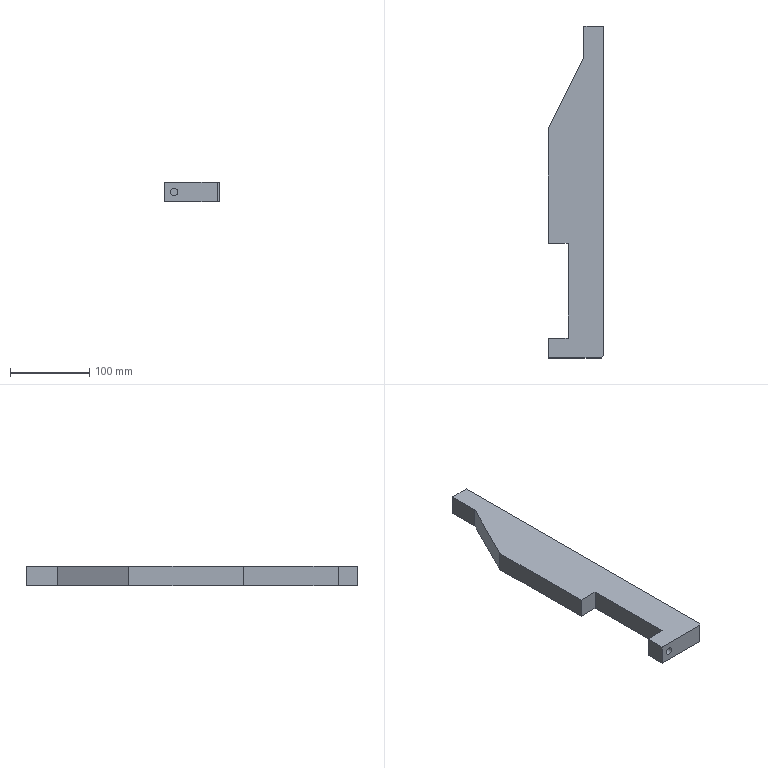CAM job | NX | 3-axis milling | part box 70 x 420 x 25 mm | stock box 75 x 425 x 30 mm
Tools:
number,name,description,diameter,corner_radius,flute_length,length,flutes
9,D10,平底铣刀-粗,10.0,0.0,35.0,75.0,2
11,D3-J,平底铣刀-精,3.0,0.0,50.0,75.0,2
7,D6-J,平底铣刀-精,6.0,0.0,25.0,75.0,2
1,D80R0.8飞刀,圆鼻刀-粗,80.0,0.8,50.0,75.0,2
1,D80R0.8飞刀-J,圆鼻刀-精,80.0,0.8,50.0,75.0,2
2,D6倒角刀,倒角刀,6.0,0.0,3.0,25.0,2
Operations:
program,operation,operation_type,tool,method,geometry_group,spindle_rpm,surface_speed,feed_per_tooth,feed_cut,feed_plunge,cut_length_mm,path_length_mm,cut_time_min,machine_time_min
B,FLOORWALL_FACE_ONEPASSROUGH_COPY,VolumeBased25DMillingOperation,D80R0.8飞刀,LAYERED-ROUGHING-DEPTHK-STEPG,W-B,2800.0,703.696,0.5357,3000.0,100.0,4753.746,9505.965,1.585,2.06
B,FLOORWALL_FACE_ONEPASSFINISH_COPY,VolumeBased25DMillingOperation,D80R0.8飞刀-J,SIDEWALL-FINISHING-DEPTHK-STEPG,W-B,4000.0,1005.28,0.125,1000.0,100.0,527.998,623.998,0.528,0.5376
B,PLANEDEBURR6X45L_COPY,SurfaceContour,D6倒角刀,CLIMBFACE_CHAMFER-DEPTH0-STEPG,W-B,6500.0,122.519,0.1154,1500.0,100.0,1002.928,1102.584,0.6686,0.6786
A,TOPFACE,FaceMilling,D80R0.8飞刀,SIDEWALL-FINISHING-DEPTHK-STEPG,W-A,4500.0,1385.0,0.1667,1500.0,100.0,1064.0,1160.0,0.7093,0.7189
A,DYNAMICROUGHD10_COPY,CavityMilling,D10,DYNAMICROUGH-DEPTHK-STEPK,W-A,8000.0,251.327,0.3125,5000.0,100.0,32276.382,33799.288,6.455,6.608
A,ZLEVELSMOOTHCORNERD3REF8_COPY,ZLevelMilling,D3-J,LAYERED-FINISHING-DEPTHK-STEPG,W-A,8000.0,75.398,0.125,2000.0,100.0,2762.74,3389.561,1.381,1.444
A,SELECTBODYONLY,SurfaceContour,D6倒角刀,METHOD,W-A,8000.0,150.796,0.1875,3000.0,100.0,1010.049,1105.85,0.3367,0.3463
A,PROFILE_SEMIFINISH_2,VolumeBased25DMillingOperation,D6-J,METHOD,W-A,9000.0,169.646,0.0667,1200.0,100.0,3045.093,3447.133,2.538,2.578